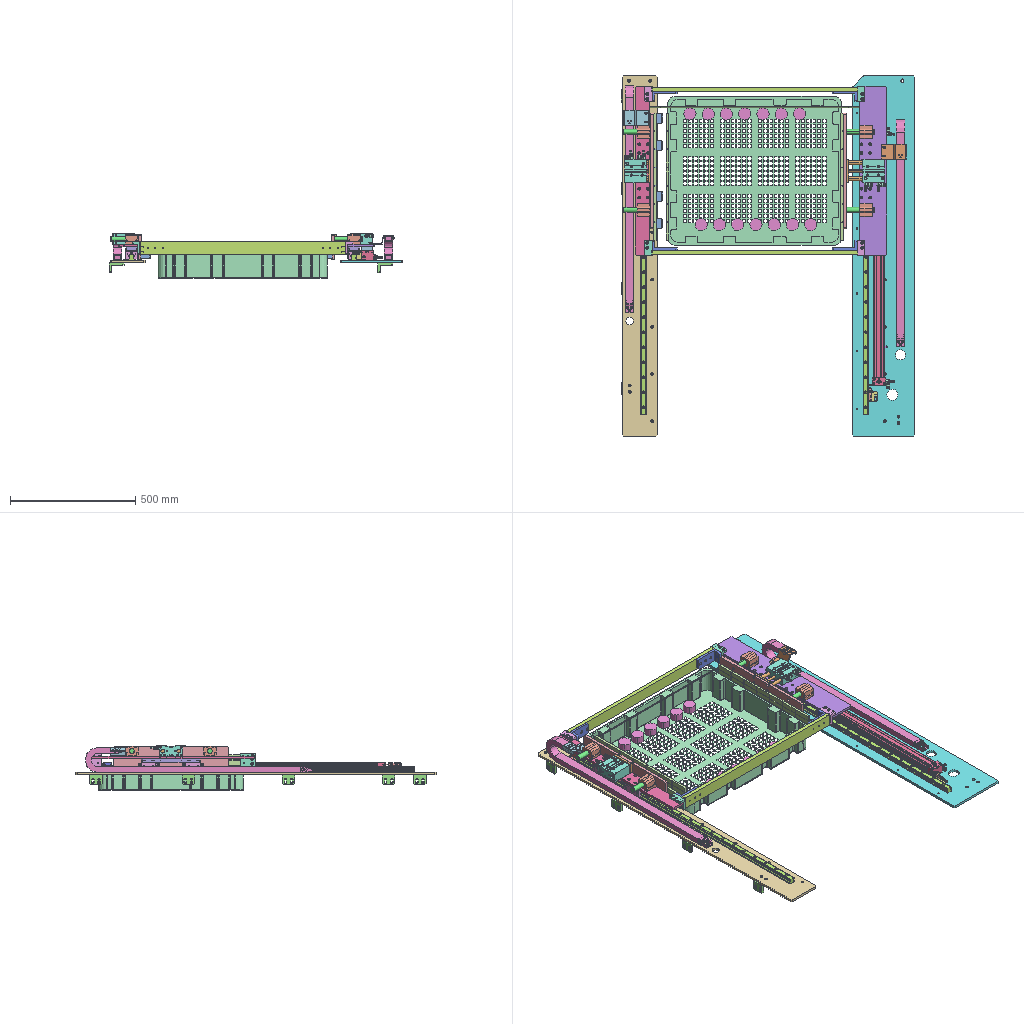Assembly | SolidWorks | 41 different items | 143 placed | box 1174 x 1440 x 177 mm
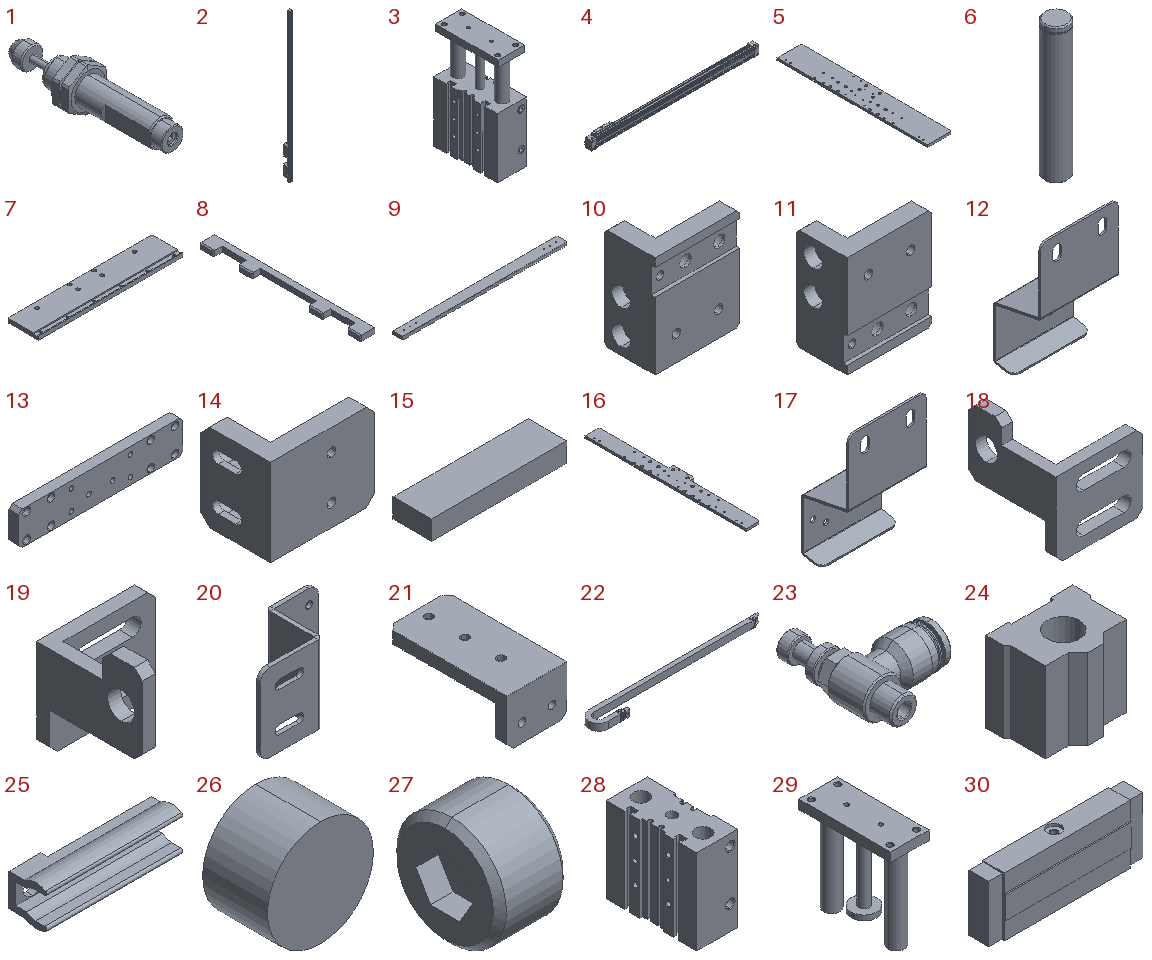Parts list (item | name | quantity | parent item | size | volume | features):
1 | (subassembly) | x2 | - | 17 x 70.5 x 19.048 mm | 7303 mm3 | -
2 | (subassembly) | x2 | - | 48 x 40 x 1200 mm | 702488 mm3 | -
3 | (subassembly) | x2 | - | 42 x 93 x 153.5 mm | 318339 mm3 | -
4 | (subassembly) | x1 | - | 1022 x 54 x 60.6 mm | 1632834 mm3 | -
5 | - | x1 | - | 108 x 675 x 10 mm | 710685 mm3 | features HoleWzd 6, Chamfer 1, Cut 1, Extrusion 1
6 | - | x4 | - | 20 x 20 x 113.5 mm | 35150 mm3 | features Chamfer 1, Extrusion 1, HoleWzd 1, RevCut 1
7 | - | x2 | - | 462 x 100 x 12 mm | 516299 mm3 | features HoleWzd 3, Chamfer 1, Cut 1, Extrusion 1, ICE 1
8 | - | x2 | - | 40.5 x 462 x 15 mm | 171000 mm3 | features Chamfer 1, Extrusion 1, HoleWzd 1
9 | - | x2 | - | 824 x 50 x 15 mm | 614536 mm3 | features HoleWzd 3, Chamfer 1, Extrusion 1, MirrorPattern 1
10 | - | x2 | - | 50 x 30 x 60 mm | 36632 mm3 | features HoleWzd 4, Chamfer 1, Extrusion 1, ICE 1
11 | - | x2 | - | 50 x 30 x 60 mm | 36632 mm3 | features HoleWzd 4, Chamfer 1, Extrusion 1, ICE 1
12 | - | x1 | - | 60 x 36.5 x 100 mm | 12211 mm3 | features Cut 1, Fillet 1, FlatPattern 1, HoleWzd 1, SMBaseFlange 1, SheetMetal 1
13 | - | x2 | - | 236 x 14 x 48 mm | 146515 mm3 | features HoleWzd 3, Chamfer 1, Extrusion 1
14 | - | x5 | - | 60 x 40 x 50 mm | 40761 mm3 | features HoleWzd 2, Chamfer 1, Extrusion 1
15 | - | x42 | - | 70 x 20 x 10 mm | 14000 mm3 | features Extrusion 1
16 | - | x1 | - | 78 x 675 x 10 mm | 392001 mm3 | features HoleWzd 7, Chamfer 1, Cut 1, Extrusion 1, ICE 1
17 | - | x1 | - | 60 x 36.5 x 100 mm | 12211 mm3 | features Cut 1, Fillet 1, FlatPattern 1, HoleWzd 1, SMBaseFlange 1, SheetMetal 1
18 | - | x1 | - | 40 x 40 x 45 mm | 9137 mm3 | features HoleWzd 2, ICE 2, Chamfer 1, Extrusion 1
19 | - | x1 | - | 40 x 40 x 45 mm | 9137 mm3 | features MirrorStock 1
20 | - | x2 | - | 55 x 27 x 40 mm | 5908 mm3 | features ICE 2, Fillet 1, FlatPattern 1, SMBaseFlange 1, SheetMetal 1
21 | - | x4 | - | 50 x 100 x 40 mm | 61642 mm3 | features HoleWzd 2, Chamfer 1, ExtruThin 1
22 | - | x2 | - | 907.2 x 99 x 35 mm | 815735 mm3 | features MoveCopyBody 4, ICE 3, Split 2, BaseBody 1
23 | - | x6 | - | 33.5 x 41.5 x 15 mm | 5376 mm3 | features BaseBody 1
24 | - | x4 | - | 54 x 41 x 50 mm | 75018 mm3 | features Extrusion 1, HoleWzd 1, LPattern 1
25 | - | x2 | in 4 | 20 x 5.565 x 5.85 mm | 175.472 mm3 | features BaseBody 1
26 | - | x14 | - | 48.94 x 30 x 48.94 mm | 56434 mm3 | features Extrusion 1
27 | - | x4 | in 3 | 6.2 x 9.728 x 9.728 mm | 415.838 mm3 | features BaseBody 1
28 | - | x2 | in 3 | 42 x 93 x 87.5 mm | 243937 mm3 | features BaseBody 1
29 | - | x2 | in 3 | 38 x 91 x 95.5 mm | 72871 mm3 | features BaseBody 1
30 | - | x1 | in 4 | 110 x 16.6 x 42 mm | 70637 mm3 | features BaseBody 1
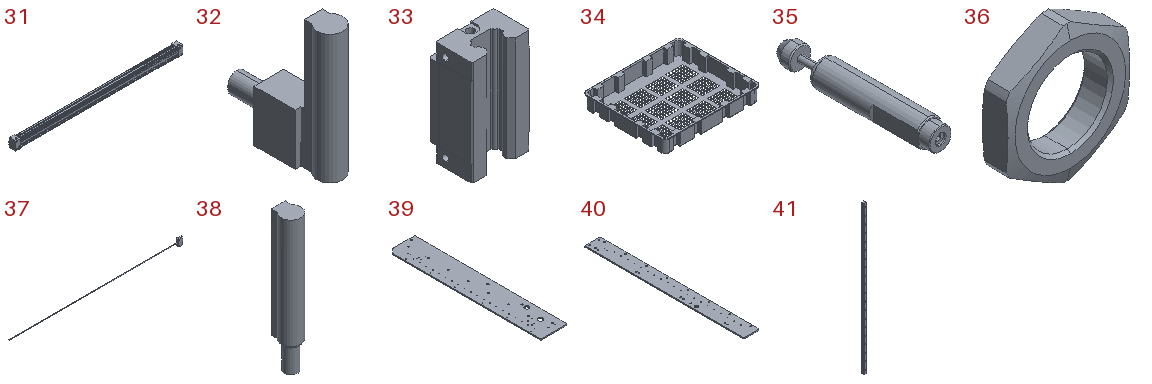31 | - | x1 | in 4 | 1022 x 40.5 x 53 mm | 1560692 mm3 | features BaseBody 1
32 | - | x2 | in 4 | 4.6 x 16.5 x 20 mm | 576.753 mm3 | features BaseBody 1
33 | - | x4 | in 2 | 48 x 34.5 x 84 mm | 100839 mm3 | features BaseBody 3
34 | - | x1 | - | 695 x 595 x 100 mm | 1469602 mm3 | features ICE 5, Fillet 3, Extrusion 1, Shell 1
35 | - | x2 | in 1 | 12 x 70.5 x 12 mm | 6151 mm3 | features BaseBody 1
36 | - | x4 | in 1 | 17 x 4 x 19.048 mm | 576.259 mm3 | features BaseBody 1
37 | - | x2 | - | 822.394 x 11.2 x 35.904 mm | 12330 mm3 | features Boss 4, Chamfer 3, Fillet 3, Cut 2, Dome 2, Extrusion 1, HoleWzd 1, ICE 1
38 | - | x4 | in 3 | 3.95 x 4.575 x 27.8 mm | 349.99 mm3 | features BaseBody 1
39 | - | x1 | - | 250 x 1440 x 10 mm | 3544237 mm3 | features HoleWzd 9, Cut 2, Chamfer 1, Extrusion 1, Fillet 1
40 | - | x1 | - | 140 x 1440 x 10 mm | 1990912 mm3 | features HoleWzd 5, Chamfer 1, Cut 1, Extrusion 1
41 | - | x2 | in 2 | 23 x 22 x 1200 mm | 500809 mm3 | features BaseBody 3
Mates (type | each side: item.copy, entity, surface, feature):
In the top assembly
Coincident | 39.1 face plane Boss-Extrude1 | 40.1 face plane Boss-Extrude1 | 2 times
DistanceDim | 40.1 face plane Boss-Extrude1 | 39.1 face plane Boss-Extrude1
Width | 5.1 face plane Boss-Extrude1 | 5.1 face plane Boss-Extrude1 | 34.1 face plane Cut-Extrude1 | 34.1 face plane Cut-Extrude1
DistanceDim | 39.1 face plane Boss-Extrude1 | 5.1 face plane Boss-Extrude1
Coincident | 5.1 face plane Boss-Extrude1 | 24.1 face plane Extrude1 | 2 times
Coincident | 5.1 face plane Boss-Extrude1 | 24.2 face plane Extrude1 | 2 times
Concentric | 24.1 face cylinder Extrude1 | 6.1 face cylinder Boss-Extrude1
Concentric | 24.2 face cylinder Extrude1 | 6.2 face cylinder Boss-Extrude1
Coincident | 6.1 face plane Boss-Extrude1 | 6.2 face plane Boss-Extrude1
Width | 5.1 face plane Boss-Extrude1 | 5.1 face plane Boss-Extrude1 | 7.1 face plane Boss-Extrude1 | 7.1 face plane Boss-Extrude1
DistanceDim | 7.1 face plane Boss-Extrude1 | 6.1 face plane Boss-Extrude1
DistanceDim | 7.1 face plane Boss-Extrude1 | 6.1 face cylinder Boss-Extrude1
Coincident | 7.1 face plane Cut-Extrude1 | 8.1 face plane Boss-Extrude1
Width | 8.1 face plane Boss-Extrude1 | 8.1 face plane Boss-Extrude1 | 7.1 face plane Boss-Extrude1 | 7.1 face plane Boss-Extrude1
Width | 8.1 face plane Boss-Extrude1 | 8.1 face plane Boss-Extrude1 | 7.1 face plane Cut-Extrude1 | 7.1 face plane Cut-Extrude1
Coincident | 40.1 face plane Boss-Extrude1 | 41.1 face plane Input1
DistanceDim | 41.1 face plane Input1 | 40.1 face plane Boss-Extrude1
Width | 8.1 face plane Boss-Extrude1 | 8.1 face plane Boss-Extrude1 | 24.1 face plane Extrude1 | 24.1 face plane Extrude1
Width | 8.1 face plane Boss-Extrude1 | 8.1 face plane Boss-Extrude1 | 24.2 face plane Extrude1 | 24.2 face plane Extrude1
Width | 7.1 face plane Boss-Extrude1 | 7.1 face plane Boss-Extrude1 | 33.1 face plane Input2 | 33.2 face plane Input2
DistanceDim | 9.1 face plane Boss-Extrude1 | 5.1 face plane Boss-Extrude1
Coincident | 24.3 face plane Extrude1 | 16.1 face plane Boss-Extrude1 | 2 times
Coincident | 24.4 face plane Extrude1 | 16.1 face plane Boss-Extrude1 | 2 times
Coincident | 6.3 face plane Boss-Extrude1 | 6.4 face plane Boss-Extrude1
Width | 8.2 face plane Boss-Extrude1 | 8.2 face plane Boss-Extrude1 | 7.2 face plane Cut-Extrude1 | 7.2 face plane Cut-Extrude1
Width | 16.1 face plane Boss-Extrude1 | 16.1 face plane Boss-Extrude1 | 7.2 face plane Boss-Extrude1 | 7.2 face plane Boss-Extrude1
Concentric | 6.4 face cylinder Boss-Extrude1 | 24.3 face cylinder Extrude1
Width | 8.2 face plane Boss-Extrude1 | 8.2 face plane Boss-Extrude1 | 7.2 face plane Boss-Extrude1 | 7.2 face plane Boss-Extrude1
Concentric | 6.3 face cylinder Boss-Extrude1 | 24.4 face cylinder Extrude1
DistanceDim | 7.2 face plane Boss-Extrude1 | 6.4 face plane Boss-Extrude1
DistanceDim | 7.2 face plane Boss-Extrude1 | 6.4 face cylinder Boss-Extrude1
Coincident | 8.2 face plane Boss-Extrude1 | 7.2 face plane Cut-Extrude1
Width | 8.2 face plane Boss-Extrude1 | 8.2 face plane Boss-Extrude1 | 24.3 face plane Extrude1 | 24.3 face plane Extrude1
Width | 8.2 face plane Boss-Extrude1 | 8.2 face plane Boss-Extrude1 | 24.4 face plane Extrude1 | 24.4 face plane Extrude1
Coincident | 5.1 face plane Boss-Extrude1 | 16.1 face plane Boss-Extrude1 | 2 times
Coincident | 40.1 face plane Boss-Extrude1 | 41.2 face plane Input1
Coincident | 41.1 face plane Input1 | 41.2 face plane Input1
DistanceDim | 16.1 face plane Boss-Extrude1 | 40.1 face plane Boss-Extrude1
DistanceDim | 41.2 face plane Input1 | 40.1 face plane Boss-Extrude1
Coincident | 9.1 face plane Boss-Extrude1 | 9.2 face plane Boss-Extrude1 | 2 times
Coincident | 39.1 face plane Boss-Extrude1 | 31.1 face plane Input1
Width | 40.1 face plane Boss-Extrude1 | 39.1 face plane Boss-Extrude1 | 34.1 face plane Cut-Extrude1 | 34.1 face plane Cut-Extrude1
Coincident | 34.1 face plane Boss-Extrude2 | 8.2 face plane Boss-Extrude1
Coincident | 5.1 face plane Boss-Extrude1 | 33.2 face plane Input2
DistanceDim | 31.1 face plane Input1 | 39.1 face plane Boss-Extrude1
DistanceDim | 5.1 face plane Boss-Extrude1 | 39.1 face plane Boss-Extrude1
Coincident | 7.1 face plane Boss-Extrude1 | 29.1 face plane Input1
DistanceDim | 28.1 face plane Input1 | 5.1 face plane Boss-Extrude1
Width | 5.1 face plane Boss-Extrude1 | 5.1 face plane Boss-Extrude1 | 28.1 face plane Input1 | 28.1 face plane Input1
DistanceDim | 39.1 face plane Boss-Extrude1 | 31.1 face plane Input1
Coincident | 5.1 face plane Boss-Extrude1 | 28.1 face plane Input1
Width | 30.1 face plane Input1 | 30.1 face plane Input1 | 28.1 face plane Input1 | 28.1 face plane Input1
Coincident | 16.1 face plane Boss-Extrude1 | 28.2 face plane Input1
Coincident | 7.2 face plane Boss-Extrude1 | 29.2 face plane Input1
Coincident | 28.1 face plane Input1 | 28.2 face plane Input1
Concentric | 31.1 face cylinder Input1 | 23.1 face cylinder Input1
Coincident | 31.1 face plane Input1 | 23.1 face plane Input1
Parallel | 31.1 face plane Input1 | 23.1 face plane Input1
Concentric | 31.1 face cylinder Input1 | 23.2 face cylinder Input1
Coincident | 31.1 face plane Input1 | 23.2 face plane Input1
Parallel | 31.1 face plane Input1 | 23.2 face plane Input1
Concentric | 28.2 face cone Input1 | 23.3 face cylinder Input1
Coincident | 28.2 face plane Input1 | 23.3 face plane Input1
Parallel | 28.2 face plane Input1 | 23.3 face plane Input1
Concentric | 28.2 face cone Input1 | 23.4 face cylinder Input1
Coincident | 28.2 face plane Input1 | 23.4 face plane Input1
Parallel | 28.2 face plane Input1 | 23.4 face plane Input1
Concentric | 28.1 face cone Input1 | 23.5 face cylinder Input1
Coincident | 28.1 face plane Input1 | 23.5 face plane Input1
Parallel | 28.1 face plane Input1 | 23.5 face plane Input1
Concentric | 28.1 face cone Input1 | 23.6 face cylinder Input1
Coincident | 28.1 face plane Input1 | 23.6 face plane Input1
Parallel | 28.1 face plane Input1 | 23.6 face plane Input1
Coincident | 5.1 face plane Boss-Extrude1 | 10.1 face plane Boss-Extrude1 | 3 times
Coincident | 16.1 face plane Boss-Extrude1 | 11.1 face plane Boss-Extrude1 | 3 times
Coincident | 16.1 face plane Boss-Extrude1 | 10.2 face plane Boss-Extrude1 | 3 times
Coincident | 5.1 face plane Boss-Extrude1 | 11.2 face plane Boss-Extrude1 | 3 times
Coincident | 39.1 face plane Boss-Extrude1 | 22.1 face plane Input1
DistanceDim | 22.1 face plane Input1 | 39.1 face plane Boss-Extrude1
Coincident | 28.1 face plane Input1 | 22.1 face plane Input1
Coincident | 5.1 face plane Boss-Extrude1 | 12.1 face plane Base-Flange1
Width | 12.1 face plane Base-Flange1 | 12.1 face plane Base-Flange1 | 22.1 face plane Input1 | 22.1 face plane Input1
Coincident | 22.1 face plane Input1 | 12.1 face plane Base-Flange1
Coincident | 33.1 face plane Input2 | 13.1 face plane Boss-Extrude1
Width | 13.1 face plane Boss-Extrude1 | 13.1 face plane Boss-Extrude1 | 33.1 face plane Input2 | 33.1 face plane Input2
Coincident | 16.1 face plane Boss-Extrude1 | 13.2 face plane Boss-Extrude1
Concentric | 9.1 face cylinder M6 Threaded Hole1 | 10.2 face cylinder M6 CBORE for Socket Head Cap Screw1
Concentric | 9.2 face cylinder M4 Threaded Hole1 | 11.1 face cylinder M4 CBORE for Socket Head Cap Screw1
Coincident | 40.1 face plane Boss-Extrude1 | 14.1 face plane Boss-Extrude1
DistanceDim | 14.1 face plane Boss-Extrude1 | 40.1 face plane Boss-Extrude1 | 2 times
Coincident | 39.1 face plane Boss-Extrude1 | 14.2 face plane Boss-Extrude1
DistanceDim | 14.2 face plane Boss-Extrude1 | 39.1 face plane Boss-Extrude1 | 2 times
DistanceDim | 34.1 face plane Cut-Extrude1 | 39.1 face plane Boss-Extrude1
Coincident | 40.1 face plane Boss-Extrude1 | 22.2 face plane Input1
Concentric | 16.1 face cylinder M5 Threaded Hole1 | 28.2 face cylinder Input1
Coincident | 22.2 face plane Input1 | 17.1 face plane Base-Flange1 | 2 times
Width | 17.1 face plane Base-Flange1 | 17.1 face plane Base-Flange1 | 22.2 face plane Input1 | 22.2 face plane Input1
DistanceDim | 22.2 face plane Input1 | 16.1 face plane Cut-Extrude2
Coincident | 24.3 face plane Extrude1 | 17.1 face plane Base-Flange1
Coincident | 39.1 face plane Boss-Extrude1 | 18.1 face plane Boss-Extrude1
Coincident | 41.1 face plane Input1 | 18.1 face plane Cut-Extrude1
Concentric | 35.1 face cylinder Input1 | 18.1 face cylinder M12 Threaded Hole1
DistanceDim | 18.1 face plane Boss-Extrude1 | 39.1 face plane Boss-Extrude1
DistanceDim | 35.1 face plane Input1 | 18.1 face plane Boss-Extrude1
Coincident | 39.1 face plane Boss-Extrude1 | 19.1 face plane
Coincident | 18.1 face plane Boss-Extrude1 | 19.1 face plane
Concentric | 35.2 face cylinder Input1 | 19.1 face cylinder
DistanceDim | 35.2 face plane Input1 | 19.1 face plane
Coincident | 31.1 face plane Input1 | 19.1 face plane
DistanceDim | 37.1 face plane Extrude1 | 39.1 face plane Boss-Extrude1 | 2 times
Concentric | 37.1 face cylinder Boss-Extrude1 | 37.2 face cylinder Boss-Extrude1
DistanceDim | 37.2 face plane Extrude1 | 40.1 face plane Boss-Extrude1
Concentric | 33.3 face cylinder Input2 | 13.2 face cylinder M6 CBORE for Socket Head Cap Screw1
Concentric | 33.4 face cylinder Input2 | 13.2 face cylinder M6 CBORE for Socket Head Cap Screw1
Width | 13.2 face plane Boss-Extrude1 | 13.2 face plane Boss-Extrude1 | 16.1 face plane Boss-Extrude1 | 16.1 face plane Boss-Extrude1
Concentric | 33.2 face cylinder Input2 | 13.1 face cylinder M6 CBORE for Socket Head Cap Screw1
Concentric | 33.1 face cylinder Input2 | 13.1 face cylinder M6 CBORE for Socket Head Cap Screw1
Coincident | 37.2 face plane Extrude1 | 37.1 face plane Extrude1
Coincident | 39.1 face plane Boss-Extrude1 | 20.1 face plane Base-Flange1
Width | 20.1 face plane Base-Flange1 | 20.1 face plane Base-Flange1 | 37.1 face plane Extrude1 | 37.1 face plane Extrude1
DistanceDim | 37.1 face plane Extrude1 | 20.1 face plane Base-Flange1
Coincident | 40.1 face plane Boss-Extrude1 | 20.2 face plane Base-Flange1
Coincident | 20.1 face plane Base-Flange1 | 20.2 face plane Base-Flange1
Concentric | 37.2 face cylinder M3x0.5 Threaded Hole1 | 20.2 face cylinder Cut-Extrude1
Coincident | 37.1 face plane Extrude1 | 20.1 face plane Base-Flange1
Coincident | 14.3 face plane Boss-Extrude1 | 14.4 face plane Boss-Extrude1
Concentric | 40.1 face cylinder M6 CBORE for Socket Head Cap Screw1 | 14.4 face cylinder M6 Threaded Hole1
Parallel | 40.1 face plane Boss-Extrude1 | 14.4 face plane Boss-Extrude1
Coincident | 11.1 face plane Boss-Extrude1 | 21.1 face plane Extrude-Thin2
Coincident | 9.2 face plane Boss-Extrude1 | 21.1 face plane Extrude-Thin2 | 2 times
Coincident | 10.1 face plane Boss-Extrude1 | 21.2 face plane Extrude-Thin2 | 2 times
Coincident | 9.2 face plane Boss-Extrude1 | 21.2 face plane Extrude-Thin2
Coincident | 11.2 face plane Boss-Extrude1 | 21.3 face plane Extrude-Thin2 | 2 times
Coincident | 9.1 face plane Boss-Extrude1 | 21.3 face plane Extrude-Thin2
Coincident | 9.1 face plane Boss-Extrude1 | 21.4 face plane Extrude-Thin2 | 2 times
Coincident | 10.2 face plane Boss-Extrude1 | 21.4 face plane Extrude-Thin2
Coincident | 7.1 face plane Boss-Extrude1 | 15.1 face plane Boss-Extrude1 | 2 times
Coincident | 34.1 face plane Boss-Extrude1 | 15.1 face plane Boss-Extrude1
Coincident | 34.1 face plane Shell1 | 26.1 face plane Boss-Extrude1
Coincident | 34.1 face plane Shell1 | 26.2 face plane Boss-Extrude1
In subassembly 3
Concentric | 28.3 face cylinder Input1 | 29.3 face cylinder Input1 | 2 times
LimitDistanceDim | 29.3 face plane Input1 | 28.3 face plane Input1
Concentric | 28.3 face cylinder Input1 | 38.1 face cylinder Input1
Parallel | 28.3 face plane Input1 | 38.1 face plane Input1
Concentric | 28.3 face cylinder Input1 | 38.2 face cylinder Input1
Parallel | 28.3 face plane Input1 | 38.2 face plane Input1
DistanceDim | 38.2 face plane Input1 | 28.3 face plane Input1
DistanceDim | 38.1 face plane Input1 | 28.3 face plane Input1
In subassembly 4
DistanceDim | 30.2 face plane Input1 | 31.2 face plane Input1 | 2 times
LimitDistanceDim | 30.2 face plane Input1 | 31.2 face plane Input1
In subassembly 2
Width | 33.5 face plane Input2 | 33.5 face plane Input2 | 41.3 face plane Input1 | 41.3 face plane Input1
Coincident | 41.3 face plane Input1 | 33.5 face plane Input2
Coincident | 33.5 face plane Input2 | 33.6 face plane Input2 | 2 times